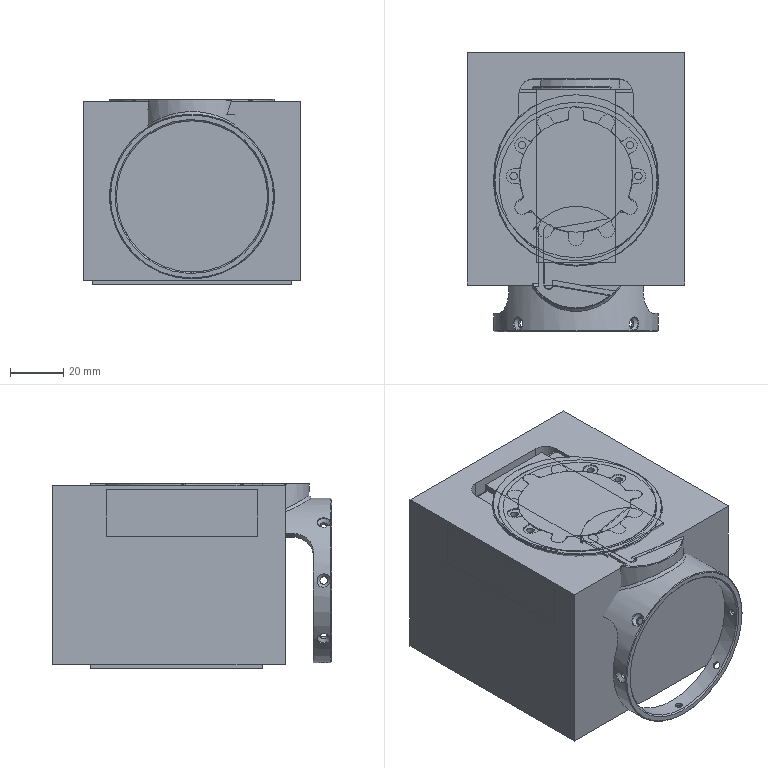NC program | NX | posted with a generic post | part box 82 x 105.2 x 70 mm
Lines 1141 to 2964 of 2964, first 1557 of 1814 lines:
(轮廓清角-D12 , TOOL : 光刀D2)
N2274 T22 M6
N2276 G53
N2278 G17 G0 G90 X21.079 Y-16.133 B0. C0. S8500 M3
N2280 G43 Z10. H22
N2282 Z-0.15
N2284 G41 G94 G1 X20.991 Y-15.953 F1000. D22
N2286 G3 X20.147 Y-15.394 R1.
N2288 G2 X18.452 Y-14.891 R3.8
N2290 G1 X17.13 Y-14.128
N2292 G2 X14.465 Y-16.822 R22.3
N2294 G3 X14.151 Y-17.854 R1.
N2296 G40
N2298 G1 X14.206 Y-18.047
N2300 G0 X21.079 Y-16.133 Z-0.3
N2302 G41 G1 X20.991 Y-15.953
N2304 G3 X20.147 Y-15.394 R1.
N2306 G2 X18.452 Y-14.891 R3.8
N2308 G1 X17.13 Y-14.128
N2310 G2 X14.465 Y-16.822 R22.3
N2312 G3 X14.151 Y-17.854 R1.
N2314 G40
N2316 G1 X14.206 Y-18.047
N2318 G0 X21.079 Y-16.133 Z-0.45
N2320 G41 G1 X20.991 Y-15.953
N2322 G3 X20.147 Y-15.394 R1.
N2324 G2 X18.452 Y-14.891 R3.8
N2326 G1 X17.13 Y-14.128
N2328 G2 X14.465 Y-16.822 R22.3
N2330 G3 X14.151 Y-17.854 R1.
N2332 G40
N2334 G1 X14.206 Y-18.047
N2336 G0 X21.079 Y-16.133 Z-0.6
N2338 G41 G1 X20.991 Y-15.953
N2340 G3 X20.147 Y-15.394 R1.
N2342 G2 X18.452 Y-14.891 R3.8
N2344 G1 X17.13 Y-14.128
N2346 G2 X14.465 Y-16.822 R22.3
N2348 G3 X14.151 Y-17.854 R1.
N2350 G40
N2352 G1 X14.206 Y-18.047
N2354 G0 X21.079 Y-16.133 Z-0.75
N2356 G41 G1 X20.991 Y-15.953
N2358 G3 X20.147 Y-15.394 R1.
N2360 G2 X18.452 Y-14.891 R3.8
N2362 G1 X17.13 Y-14.128
N2364 G2 X14.465 Y-16.822 R22.3
N2366 G3 X14.151 Y-17.854 R1.
N2368 G40
N2370 G1 X14.206 Y-18.047
N2372 G0 X21.079 Y-16.133 Z-0.9
N2374 G41 G1 X20.991 Y-15.953
N2376 G3 X20.147 Y-15.394 R1.
N2378 G2 X18.452 Y-14.891 R3.8
N2380 G1 X17.13 Y-14.128
N2382 G2 X14.465 Y-16.822 R22.3
N2384 G3 X14.151 Y-17.854 R1.
N2386 G40
N2388 G1 X14.206 Y-18.047
N2390 G0 X21.079 Y-16.133 Z-1.05
N2392 G41 G1 X20.991 Y-15.953
N2394 G3 X20.147 Y-15.394 R1.
N2396 G2 X18.452 Y-14.891 R3.8
N2398 G1 X17.13 Y-14.128
N2400 G2 X14.465 Y-16.822 R22.3
N2402 G3 X14.151 Y-17.854 R1.
N2404 G40
N2406 G1 X14.206 Y-18.047
N2408 G0 X21.079 Y-16.133 Z-1.2
N2410 G41 G1 X20.991 Y-15.953
N2412 G3 X20.147 Y-15.394 R1.
N2414 G2 X18.452 Y-14.891 R3.8
N2416 G1 X17.13 Y-14.128
N2418 G2 X14.465 Y-16.822 R22.3
N2420 G3 X14.151 Y-17.854 R1.
N2422 G40
N2424 G1 X14.206 Y-18.047
N2426 G0 X21.079 Y-16.133 Z-1.35
N2428 G41 G1 X20.991 Y-15.953
N2430 G3 X20.147 Y-15.394 R1.
N2432 G2 X18.452 Y-14.891 R3.8
N2434 G1 X17.13 Y-14.128
N2436 G2 X14.465 Y-16.822 R22.3
N2438 G3 X14.151 Y-17.854 R1.
N2440 G40
N2442 G1 X14.206 Y-18.047
N2444 G0 X21.079 Y-16.133 Z-1.5
N2446 G41 G1 X20.991 Y-15.953
N2448 G3 X20.147 Y-15.394 R1.
N2450 G2 X18.452 Y-14.891 R3.8
N2452 G1 X17.13 Y-14.128
N2454 G2 X14.465 Y-16.822 R22.3
N2456 G3 X14.151 Y-17.854 R1.
N2458 G40
N2460 G1 X14.206 Y-18.047
N2462 G0 X21.079 Y-16.133 Z-1.65
N2464 G41 G1 X20.991 Y-15.953
N2466 G3 X20.147 Y-15.394 R1.
N2468 G2 X18.452 Y-14.891 R3.8
N2470 G1 X17.13 Y-14.128
N2472 G2 X14.465 Y-16.822 R22.3
N2474 G3 X14.151 Y-17.854 R1.
N2476 G40
N2478 G1 X14.206 Y-18.047
N2480 G0 X21.079 Y-16.133 Z-1.8
N2482 G41 G1 X20.991 Y-15.953
N2484 G3 X20.147 Y-15.394 R1.
N2486 G2 X18.452 Y-14.891 R3.8
N2488 G1 X17.13 Y-14.128
N2490 G2 X14.465 Y-16.822 R22.3
N2492 G3 X14.151 Y-17.854 R1.
N2494 G40
N2496 G1 X14.206 Y-18.047
N2498 G0 X21.079 Y-16.133 Z-1.95
N2500 G41 G1 X20.991 Y-15.953
N2502 G3 X20.147 Y-15.394 R1.
N2504 G2 X18.452 Y-14.891 R3.8
N2506 G1 X17.13 Y-14.128
N2508 G2 X14.465 Y-16.822 R22.3
N2510 G3 X14.151 Y-17.854 R1.
N2512 G40
N2514 G1 X14.206 Y-18.047
N2516 G0 X21.079 Y-16.133 Z-2.1
N2518 G41 G1 X20.991 Y-15.953
N2520 G3 X20.147 Y-15.394 R1.
N2522 G2 X18.452 Y-14.891 R3.8
N2524 G1 X17.13 Y-14.128
N2526 G2 X14.465 Y-16.822 R22.3
N2528 G3 X14.151 Y-17.854 R1.
N2530 G40
N2532 G1 X14.206 Y-18.047
N2534 G0 X21.079 Y-16.133 Z-2.25
N2536 G41 G1 X20.991 Y-15.953
N2538 G3 X20.147 Y-15.394 R1.
N2540 G2 X18.452 Y-14.891 R3.8
N2542 G1 X17.13 Y-14.128
N2544 G2 X14.465 Y-16.822 R22.3
N2546 G3 X14.151 Y-17.854 R1.
N2548 G40
N2550 G1 X14.206 Y-18.047
N2552 G0 X21.079 Y-16.133 Z-2.4
N2554 G41 G1 X20.991 Y-15.953
N2556 G3 X20.147 Y-15.394 R1.
N2558 G2 X18.452 Y-14.891 R3.8
N2560 G1 X17.13 Y-14.128
N2562 G2 X14.465 Y-16.822 R22.3
N2564 G3 X14.151 Y-17.854 R1.
N2566 G40
N2568 G1 X14.206 Y-18.047
N2570 G0 X21.079 Y-16.133 Z-2.45
N2572 G41 G1 X20.991 Y-15.953
N2574 G3 X20.147 Y-15.394 R1.
N2576 G2 X18.452 Y-14.891 R3.8
N2578 G1 X17.13 Y-14.128
N2580 G2 X14.465 Y-16.822 R22.3
N2582 G3 X14.151 Y-17.854 R1.
N2584 G40
N2586 G1 X14.206 Y-18.047
N2588 G0 Z10.
N2590 X22.862 Y-3.054
N2592 Z-0.15
N2594 G41 G1 X22.668 Y-3.103
N2596 G3 X21.931 Y-3.891 R1.
N2598 G2 X20.93 Y-7.546 R22.3
N2600 G1 X22.252 Y-8.309
N2602 G2 X23.535 Y-9.526 R3.8
N2604 G3 X24.442 Y-9.977 R1.
N2606 G40
N2608 G1 X24.641 Y-9.964
N2610 G0 X22.862 Y-3.054 Z-0.3
N2612 G41 G1 X22.668 Y-3.103
N2614 G3 X21.931 Y-3.891 R1.
N2616 G2 X20.93 Y-7.546 R22.3
N2618 G1 X22.252 Y-8.309
N2620 G2 X23.535 Y-9.526 R3.8
N2622 G3 X24.442 Y-9.977 R1.
N2624 G40
N2626 G1 X24.641 Y-9.964
N2628 G0 X22.862 Y-3.054 Z-0.45
N2630 G41 G1 X22.668 Y-3.103
N2632 G3 X21.931 Y-3.891 R1.
N2634 G2 X20.93 Y-7.546 R22.3
N2636 G1 X22.252 Y-8.309
N2638 G2 X23.535 Y-9.526 R3.8
N2640 G3 X24.442 Y-9.977 R1.
N2642 G40
N2644 G1 X24.641 Y-9.964
N2646 G0 X22.862 Y-3.054 Z-0.6
N2648 G41 G1 X22.668 Y-3.103
N2650 G3 X21.931 Y-3.891 R1.
N2652 G2 X20.93 Y-7.546 R22.3
N2654 G1 X22.252 Y-8.309
N2656 G2 X23.535 Y-9.526 R3.8
N2658 G3 X24.442 Y-9.977 R1.
N2660 G40
N2662 G1 X24.641 Y-9.964
N2664 G0 X22.862 Y-3.054 Z-0.75
N2666 G41 G1 X22.668 Y-3.103
N2668 G3 X21.931 Y-3.891 R1.
N2670 G2 X20.93 Y-7.546 R22.3
N2672 G1 X22.252 Y-8.309
N2674 G2 X23.535 Y-9.526 R3.8
N2676 G3 X24.442 Y-9.977 R1.
N2678 G40
N2680 G1 X24.641 Y-9.964
N2682 G0 X22.862 Y-3.054 Z-0.9
N2684 G41 G1 X22.668 Y-3.103
N2686 G3 X21.931 Y-3.891 R1.
N2688 G2 X20.93 Y-7.546 R22.3
N2690 G1 X22.252 Y-8.309
N2692 G2 X23.535 Y-9.526 R3.8
N2694 G3 X24.442 Y-9.977 R1.
N2696 G40
N2698 G1 X24.641 Y-9.964
N2700 G0 X22.862 Y-3.054 Z-1.05
N2702 G41 G1 X22.668 Y-3.103
N2704 G3 X21.931 Y-3.891 R1.
N2706 G2 X20.93 Y-7.546 R22.3
N2708 G1 X22.252 Y-8.309
N2710 G2 X23.535 Y-9.526 R3.8
N2712 G3 X24.442 Y-9.977 R1.
N2714 G40
N2716 G1 X24.641 Y-9.964
N2718 G0 X22.862 Y-3.054 Z-1.2
N2720 G41 G1 X22.668 Y-3.103
N2722 G3 X21.931 Y-3.891 R1.
N2724 G2 X20.93 Y-7.546 R22.3
N2726 G1 X22.252 Y-8.309
N2728 G2 X23.535 Y-9.526 R3.8
N2730 G3 X24.442 Y-9.977 R1.
N2732 G40
N2734 G1 X24.641 Y-9.964
N2736 G0 X22.862 Y-3.054 Z-1.35
N2738 G41 G1 X22.668 Y-3.103
N2740 G3 X21.931 Y-3.891 R1.
N2742 G2 X20.93 Y-7.546 R22.3
N2744 G1 X22.252 Y-8.309
N2746 G2 X23.535 Y-9.526 R3.8
N2748 G3 X24.442 Y-9.977 R1.
N2750 G40
N2752 G1 X24.641 Y-9.964
N2754 G0 X22.862 Y-3.054 Z-1.5
N2756 G41 G1 X22.668 Y-3.103
N2758 G3 X21.931 Y-3.891 R1.
N2760 G2 X20.93 Y-7.546 R22.3
N2762 G1 X22.252 Y-8.309
N2764 G2 X23.535 Y-9.526 R3.8
N2766 G3 X24.442 Y-9.977 R1.
N2768 G40
N2770 G1 X24.641 Y-9.964
N2772 G0 X22.862 Y-3.054 Z-1.65
N2774 G41 G1 X22.668 Y-3.103
N2776 G3 X21.931 Y-3.891 R1.
N2778 G2 X20.93 Y-7.546 R22.3
N2780 G1 X22.252 Y-8.309
N2782 G2 X23.535 Y-9.526 R3.8
N2784 G3 X24.442 Y-9.977 R1.
N2786 G40
N2788 G1 X24.641 Y-9.964
N2790 G0 X22.862 Y-3.054 Z-1.8
N2792 G41 G1 X22.668 Y-3.103
N2794 G3 X21.931 Y-3.891 R1.
N2796 G2 X20.93 Y-7.546 R22.3
N2798 G1 X22.252 Y-8.309
N2800 G2 X23.535 Y-9.526 R3.8
N2802 G3 X24.442 Y-9.977 R1.
N2804 G40
N2806 G1 X24.641 Y-9.964
N2808 G0 X22.862 Y-3.054 Z-1.95
N2810 G41 G1 X22.668 Y-3.103
N2812 G3 X21.931 Y-3.891 R1.
N2814 G2 X20.93 Y-7.546 R22.3
N2816 G1 X22.252 Y-8.309
N2818 G2 X23.535 Y-9.526 R3.8
N2820 G3 X24.442 Y-9.977 R1.
N2822 G40
N2824 G1 X24.641 Y-9.964
N2826 G0 X22.862 Y-3.054 Z-2.1
N2828 G41 G1 X22.668 Y-3.103
N2830 G3 X21.931 Y-3.891 R1.
N2832 G2 X20.93 Y-7.546 R22.3
N2834 G1 X22.252 Y-8.309
N2836 G2 X23.535 Y-9.526 R3.8
N2838 G3 X24.442 Y-9.977 R1.
N2840 G40
N2842 G1 X24.641 Y-9.964
N2844 G0 X22.862 Y-3.054 Z-2.25
N2846 G41 G1 X22.668 Y-3.103
N2848 G3 X21.931 Y-3.891 R1.
N2850 G2 X20.93 Y-7.546 R22.3
N2852 G1 X22.252 Y-8.309
N2854 G2 X23.535 Y-9.526 R3.8
N2856 G3 X24.442 Y-9.977 R1.
N2858 G40
N2860 G1 X24.641 Y-9.964
N2862 G0 X22.862 Y-3.054 Z-2.4
N2864 G41 G1 X22.668 Y-3.103
N2866 G3 X21.931 Y-3.891 R1.
N2868 G2 X20.93 Y-7.546 R22.3
N2870 G1 X22.252 Y-8.309
N2872 G2 X23.535 Y-9.526 R3.8
N2874 G3 X24.442 Y-9.977 R1.
N2876 G40
N2878 G1 X24.641 Y-9.964
N2880 G0 X22.862 Y-3.054 Z-2.45
N2882 G41 G1 X22.668 Y-3.103
N2884 G3 X21.931 Y-3.891 R1.
N2886 G2 X20.93 Y-7.546 R22.3
N2888 G1 X22.252 Y-8.309
N2890 G2 X23.535 Y-9.526 R3.8
N2892 G3 X24.442 Y-9.977 R1.
N2894 G40
N2896 G1 X24.641 Y-9.964
N2898 G0 Z10.
N2900 X3.562 Y26.547
N2902 Z-0.15
N2904 G41 G1 X3.45 Y26.381
N2906 G3 X3.388 Y25.37 R1.
N2908 G2 X3.8 Y23.65 R3.8
N2910 G1 Y22.124
N2912 G2 X7.466 Y21.163 R22.3
N2914 G3 X8.516 Y21.408 R1.
N2916 G40
N2918 G1 X8.656 Y21.551
N2920 G0 X3.562 Y26.547 Z-0.3
N2922 G41 G1 X3.45 Y26.381
N2924 G3 X3.388 Y25.37 R1.
N2926 G2 X3.8 Y23.65 R3.8
N2928 G1 Y22.124
N2930 G2 X7.466 Y21.163 R22.3
N2932 G3 X8.516 Y21.408 R1.
N2934 G40
N2936 G1 X8.656 Y21.551
N2938 G0 X3.562 Y26.547 Z-0.45
N2940 G41 G1 X3.45 Y26.381
N2942 G3 X3.388 Y25.37 R1.
N2944 G2 X3.8 Y23.65 R3.8
N2946 G1 Y22.124
N2948 G2 X7.466 Y21.163 R22.3
N2950 G3 X8.516 Y21.408 R1.
N2952 G40
N2954 G1 X8.656 Y21.551
N2956 G0 X3.562 Y26.547 Z-0.6
N2958 G41 G1 X3.45 Y26.381
N2960 G3 X3.388 Y25.37 R1.
N2962 G2 X3.8 Y23.65 R3.8
N2964 G1 Y22.124
N2966 G2 X7.466 Y21.163 R22.3
N2968 G3 X8.516 Y21.408 R1.
N2970 G40
N2972 G1 X8.656 Y21.551
N2974 G0 X3.562 Y26.547 Z-0.75
N2976 G41 G1 X3.45 Y26.381
N2978 G3 X3.388 Y25.37 R1.
N2980 G2 X3.8 Y23.65 R3.8
N2982 G1 Y22.124
N2984 G2 X7.466 Y21.163 R22.3
N2986 G3 X8.516 Y21.408 R1.
N2988 G40
N2990 G1 X8.656 Y21.551
N2992 G0 X3.562 Y26.547 Z-0.9
N2994 G41 G1 X3.45 Y26.381
N2996 G3 X3.388 Y25.37 R1.
N2998 G2 X3.8 Y23.65 R3.8
N3000 G1 Y22.124
N3002 G2 X7.466 Y21.163 R22.3
N3004 G3 X8.516 Y21.408 R1.
N3006 G40
N3008 G1 X8.656 Y21.551
N3010 G0 X3.562 Y26.547 Z-1.05
N3012 G41 G1 X3.45 Y26.381
N3014 G3 X3.388 Y25.37 R1.
N3016 G2 X3.8 Y23.65 R3.8
N3018 G1 Y22.124
N3020 G2 X7.466 Y21.163 R22.3
N3022 G3 X8.516 Y21.408 R1.
N3024 G40
N3026 G1 X8.656 Y21.551
N3028 G0 X3.562 Y26.547 Z-1.2
N3030 G41 G1 X3.45 Y26.381
N3032 G3 X3.388 Y25.37 R1.
N3034 G2 X3.8 Y23.65 R3.8
N3036 G1 Y22.124
N3038 G2 X7.466 Y21.163 R22.3
N3040 G3 X8.516 Y21.408 R1.
N3042 G40
N3044 G1 X8.656 Y21.551
N3046 G0 X3.562 Y26.547 Z-1.35
N3048 G41 G1 X3.45 Y26.381
N3050 G3 X3.388 Y25.37 R1.
N3052 G2 X3.8 Y23.65 R3.8
N3054 G1 Y22.124
N3056 G2 X7.466 Y21.163 R22.3
N3058 G3 X8.516 Y21.408 R1.
N3060 G40
N3062 G1 X8.656 Y21.551
N3064 G0 X3.562 Y26.547 Z-1.5
N3066 G41 G1 X3.45 Y26.381
N3068 G3 X3.388 Y25.37 R1.
N3070 G2 X3.8 Y23.65 R3.8
N3072 G1 Y22.124
N3074 G2 X7.466 Y21.163 R22.3
N3076 G3 X8.516 Y21.408 R1.
N3078 G40
N3080 G1 X8.656 Y21.551
N3082 G0 X3.562 Y26.547 Z-1.65
N3084 G41 G1 X3.45 Y26.381
N3086 G3 X3.388 Y25.37 R1.
N3088 G2 X3.8 Y23.65 R3.8
N3090 G1 Y22.124
N3092 G2 X7.466 Y21.163 R22.3
N3094 G3 X8.516 Y21.408 R1.
N3096 G40
N3098 G1 X8.656 Y21.551
N3100 G0 X3.562 Y26.547 Z-1.8
N3102 G41 G1 X3.45 Y26.381
N3104 G3 X3.388 Y25.37 R1.
N3106 G2 X3.8 Y23.65 R3.8
N3108 G1 Y22.124
N3110 G2 X7.466 Y21.163 R22.3
N3112 G3 X8.516 Y21.408 R1.
N3114 G40
N3116 G1 X8.656 Y21.551
N3118 G0 X3.562 Y26.547 Z-1.95
N3120 G41 G1 X3.45 Y26.381
N3122 G3 X3.388 Y25.37 R1.
N3124 G2 X3.8 Y23.65 R3.8
N3126 G1 Y22.124
N3128 G2 X7.466 Y21.163 R22.3
N3130 G3 X8.516 Y21.408 R1.
N3132 G40
N3134 G1 X8.656 Y21.551
N3136 G0 X3.562 Y26.547 Z-2.1
N3138 G41 G1 X3.45 Y26.381
N3140 G3 X3.388 Y25.37 R1.
N3142 G2 X3.8 Y23.65 R3.8
N3144 G1 Y22.124
N3146 G2 X7.466 Y21.163 R22.3
N3148 G3 X8.516 Y21.408 R1.
N3150 G40
N3152 G1 X8.656 Y21.551
N3154 G0 X3.562 Y26.547 Z-2.25
N3156 G41 G1 X3.45 Y26.381
N3158 G3 X3.388 Y25.37 R1.
N3160 G2 X3.8 Y23.65 R3.8
N3162 G1 Y22.124
N3164 G2 X7.466 Y21.163 R22.3
N3166 G3 X8.516 Y21.408 R1.
N3168 G40
N3170 G1 X8.656 Y21.551
N3172 G0 X3.562 Y26.547 Z-2.4
N3174 G41 G1 X3.45 Y26.381
N3176 G3 X3.388 Y25.37 R1.
N3178 G2 X3.8 Y23.65 R3.8
N3180 G1 Y22.124
N3182 G2 X7.466 Y21.163 R22.3
N3184 G3 X8.516 Y21.408 R1.
N3186 G40
N3188 G1 X8.656 Y21.551
N3190 G0 X3.562 Y26.547 Z-2.45
N3192 G41 G1 X3.45 Y26.381
N3194 G3 X3.388 Y25.37 R1.
N3196 G2 X3.8 Y23.65 R3.8
N3198 G1 Y22.124
N3200 G2 X7.466 Y21.163 R22.3
N3202 G3 X8.516 Y21.408 R1.
N3204 G40
N3206 G1 X8.656 Y21.551
N3208 G0 Z10.
N3210 X-8.656
N3212 Z-0.15
N3214 G41 G1 X-8.516 Y21.408
N3216 G3 X-7.466 Y21.163 R1.
N3218 G2 X-3.8 Y22.124 R22.3
N3220 G1 Y23.65
N3222 G2 X-3.388 Y25.37 R3.8
N3224 G3 X-3.45 Y26.381 R1.
N3226 G40
N3228 G1 X-3.562 Y26.547
N3230 G0 X-8.656 Y21.551 Z-0.3
N3232 G41 G1 X-8.516 Y21.408
N3234 G3 X-7.466 Y21.163 R1.
N3236 G2 X-3.8 Y22.124 R22.3
N3238 G1 Y23.65
N3240 G2 X-3.388 Y25.37 R3.8
N3242 G3 X-3.45 Y26.381 R1.
N3244 G40
N3246 G1 X-3.562 Y26.547
N3248 G0 X-8.656 Y21.551 Z-0.45
N3250 G41 G1 X-8.516 Y21.408
N3252 G3 X-7.466 Y21.163 R1.
N3254 G2 X-3.8 Y22.124 R22.3
N3256 G1 Y23.65
N3258 G2 X-3.388 Y25.37 R3.8
N3260 G3 X-3.45 Y26.381 R1.
N3262 G40
N3264 G1 X-3.562 Y26.547
N3266 G0 X-8.656 Y21.551 Z-0.6
N3268 G41 G1 X-8.516 Y21.408
N3270 G3 X-7.466 Y21.163 R1.
N3272 G2 X-3.8 Y22.124 R22.3
N3274 G1 Y23.65
N3276 G2 X-3.388 Y25.37 R3.8
N3278 G3 X-3.45 Y26.381 R1.
N3280 G40
N3282 G1 X-3.562 Y26.547
N3284 G0 X-8.656 Y21.551 Z-0.75
N3286 G41 G1 X-8.516 Y21.408
N3288 G3 X-7.466 Y21.163 R1.
N3290 G2 X-3.8 Y22.124 R22.3
N3292 G1 Y23.65
N3294 G2 X-3.388 Y25.37 R3.8
N3296 G3 X-3.45 Y26.381 R1.
N3298 G40
N3300 G1 X-3.562 Y26.547
N3302 G0 X-8.656 Y21.551 Z-0.9
N3304 G41 G1 X-8.516 Y21.408
N3306 G3 X-7.466 Y21.163 R1.
N3308 G2 X-3.8 Y22.124 R22.3
N3310 G1 Y23.65
N3312 G2 X-3.388 Y25.37 R3.8
N3314 G3 X-3.45 Y26.381 R1.
N3316 G40
N3318 G1 X-3.562 Y26.547
N3320 G0 X-8.656 Y21.551 Z-1.05
N3322 G41 G1 X-8.516 Y21.408
N3324 G3 X-7.466 Y21.163 R1.
N3326 G2 X-3.8 Y22.124 R22.3
N3328 G1 Y23.65
N3330 G2 X-3.388 Y25.37 R3.8
N3332 G3 X-3.45 Y26.381 R1.
N3334 G40
N3336 G1 X-3.562 Y26.547
N3338 G0 X-8.656 Y21.551 Z-1.2
N3340 G41 G1 X-8.516 Y21.408
N3342 G3 X-7.466 Y21.163 R1.
N3344 G2 X-3.8 Y22.124 R22.3
N3346 G1 Y23.65
N3348 G2 X-3.388 Y25.37 R3.8
N3350 G3 X-3.45 Y26.381 R1.
N3352 G40
N3354 G1 X-3.562 Y26.547
N3356 G0 X-8.656 Y21.551 Z-1.35
N3358 G41 G1 X-8.516 Y21.408
N3360 G3 X-7.466 Y21.163 R1.
N3362 G2 X-3.8 Y22.124 R22.3
N3364 G1 Y23.65
N3366 G2 X-3.388 Y25.37 R3.8
N3368 G3 X-3.45 Y26.381 R1.
N3370 G40
N3372 G1 X-3.562 Y26.547
N3374 G0 X-8.656 Y21.551 Z-1.5
N3376 G41 G1 X-8.516 Y21.408
N3378 G3 X-7.466 Y21.163 R1.
N3380 G2 X-3.8 Y22.124 R22.3
N3382 G1 Y23.65
N3384 G2 X-3.388 Y25.37 R3.8
N3386 G3 X-3.45 Y26.381 R1.
N3388 G40
N3390 G1 X-3.562 Y26.547
N3392 G0 X-8.656 Y21.551 Z-1.65
N3394 G41 G1 X-8.516 Y21.408
N3396 G3 X-7.466 Y21.163 R1.
N3398 G2 X-3.8 Y22.124 R22.3
N3400 G1 Y23.65
N3402 G2 X-3.388 Y25.37 R3.8
N3404 G3 X-3.45 Y26.381 R1.
N3406 G40
N3408 G1 X-3.562 Y26.547
N3410 G0 X-8.656 Y21.551 Z-1.8
N3412 G41 G1 X-8.516 Y21.408
N3414 G3 X-7.466 Y21.163 R1.
N3416 G2 X-3.8 Y22.124 R22.3
N3418 G1 Y23.65
N3420 G2 X-3.388 Y25.37 R3.8
N3422 G3 X-3.45 Y26.381 R1.
N3424 G40
N3426 G1 X-3.562 Y26.547
N3428 G0 X-8.656 Y21.551 Z-1.95
N3430 G41 G1 X-8.516 Y21.408
N3432 G3 X-7.466 Y21.163 R1.
N3434 G2 X-3.8 Y22.124 R22.3
N3436 G1 Y23.65
N3438 G2 X-3.388 Y25.37 R3.8
N3440 G3 X-3.45 Y26.381 R1.
N3442 G40
N3444 G1 X-3.562 Y26.547
N3446 G0 X-8.656 Y21.551 Z-2.1
N3448 G41 G1 X-8.516 Y21.408
N3450 G3 X-7.466 Y21.163 R1.
N3452 G2 X-3.8 Y22.124 R22.3
N3454 G1 Y23.65
N3456 G2 X-3.388 Y25.37 R3.8
N3458 G3 X-3.45 Y26.381 R1.
N3460 G40
N3462 G1 X-3.562 Y26.547
N3464 G0 X-8.656 Y21.551 Z-2.25
N3466 G41 G1 X-8.516 Y21.408
N3468 G3 X-7.466 Y21.163 R1.
N3470 G2 X-3.8 Y22.124 R22.3
N3472 G1 Y23.65
N3474 G2 X-3.388 Y25.37 R3.8
N3476 G3 X-3.45 Y26.381 R1.
N3478 G40
N3480 G1 X-3.562 Y26.547
N3482 G0 X-8.656 Y21.551 Z-2.4
N3484 G41 G1 X-8.516 Y21.408
N3486 G3 X-7.466 Y21.163 R1.
N3488 G2 X-3.8 Y22.124 R22.3
N3490 G1 Y23.65
N3492 G2 X-3.388 Y25.37 R3.8
N3494 G3 X-3.45 Y26.381 R1.
N3496 G40
N3498 G1 X-3.562 Y26.547
N3500 G0 X-8.656 Y21.551 Z-2.45
N3502 G41 G1 X-8.516 Y21.408
N3504 G3 X-7.466 Y21.163 R1.
N3506 G2 X-3.8 Y22.124 R22.3
N3508 G1 Y23.65
N3510 G2 X-3.388 Y25.37 R3.8
N3512 G3 X-3.45 Y26.381 R1.
N3514 G40
N3516 G1 X-3.562 Y26.547
N3518 G0 Z10.
N3520 X-24.641 Y-9.964
N3522 Z-0.15
N3524 G41 G1 X-24.442 Y-9.977
N3526 G3 X-23.535 Y-9.526 R1.
N3528 G2 X-22.252 Y-8.309 R3.8
N3530 G1 X-20.93 Y-7.546
N3532 G2 X-21.931 Y-3.891 R22.3
N3534 G3 X-22.668 Y-3.103 R1.
N3536 G40
N3538 G1 X-22.862 Y-3.054
N3540 G0 X-24.641 Y-9.964 Z-0.3
N3542 G41 G1 X-24.442 Y-9.977
N3544 G3 X-23.535 Y-9.526 R1.
N3546 G2 X-22.252 Y-8.309 R3.8
N3548 G1 X-20.93 Y-7.546
N3550 G2 X-21.931 Y-3.891 R22.3
N3552 G3 X-22.668 Y-3.103 R1.
N3554 G40
N3556 G1 X-22.862 Y-3.054
N3558 G0 X-24.641 Y-9.964 Z-0.45
N3560 G41 G1 X-24.442 Y-9.977
N3562 G3 X-23.535 Y-9.526 R1.
N3564 G2 X-22.252 Y-8.309 R3.8
N3566 G1 X-20.93 Y-7.546
N3568 G2 X-21.931 Y-3.891 R22.3
N3570 G3 X-22.668 Y-3.103 R1.
N3572 G40
N3574 G1 X-22.862 Y-3.054
N3576 G0 X-24.641 Y-9.964 Z-0.6
N3578 G41 G1 X-24.442 Y-9.977
N3580 G3 X-23.535 Y-9.526 R1.
N3582 G2 X-22.252 Y-8.309 R3.8
N3584 G1 X-20.93 Y-7.546
N3586 G2 X-21.931 Y-3.891 R22.3
N3588 G3 X-22.668 Y-3.103 R1.
N3590 G40
N3592 G1 X-22.862 Y-3.054
N3594 G0 X-24.641 Y-9.964 Z-0.75
N3596 G41 G1 X-24.442 Y-9.977
N3598 G3 X-23.535 Y-9.526 R1.
N3600 G2 X-22.252 Y-8.309 R3.8
N3602 G1 X-20.93 Y-7.546
N3604 G2 X-21.931 Y-3.891 R22.3
N3606 G3 X-22.668 Y-3.103 R1.
N3608 G40
N3610 G1 X-22.862 Y-3.054
N3612 G0 X-24.641 Y-9.964 Z-0.9
N3614 G41 G1 X-24.442 Y-9.977
N3616 G3 X-23.535 Y-9.526 R1.
N3618 G2 X-22.252 Y-8.309 R3.8
N3620 G1 X-20.93 Y-7.546
N3622 G2 X-21.931 Y-3.891 R22.3
N3624 G3 X-22.668 Y-3.103 R1.
N3626 G40
N3628 G1 X-22.862 Y-3.054
N3630 G0 X-24.641 Y-9.964 Z-1.05
N3632 G41 G1 X-24.442 Y-9.977
N3634 G3 X-23.535 Y-9.526 R1.
N3636 G2 X-22.252 Y-8.309 R3.8
N3638 G1 X-20.93 Y-7.546
N3640 G2 X-21.931 Y-3.891 R22.3
N3642 G3 X-22.668 Y-3.103 R1.
N3644 G40
N3646 G1 X-22.862 Y-3.054
N3648 G0 X-24.641 Y-9.964 Z-1.2
N3650 G41 G1 X-24.442 Y-9.977
N3652 G3 X-23.535 Y-9.526 R1.
N3654 G2 X-22.252 Y-8.309 R3.8
N3656 G1 X-20.93 Y-7.546
N3658 G2 X-21.931 Y-3.891 R22.3
N3660 G3 X-22.668 Y-3.103 R1.
N3662 G40
N3664 G1 X-22.862 Y-3.054
N3666 G0 X-24.641 Y-9.964 Z-1.35
N3668 G41 G1 X-24.442 Y-9.977
N3670 G3 X-23.535 Y-9.526 R1.
N3672 G2 X-22.252 Y-8.309 R3.8
N3674 G1 X-20.93 Y-7.546
N3676 G2 X-21.931 Y-3.891 R22.3
N3678 G3 X-22.668 Y-3.103 R1.
N3680 G40
N3682 G1 X-22.862 Y-3.054
N3684 G0 X-24.641 Y-9.964 Z-1.5
N3686 G41 G1 X-24.442 Y-9.977
N3688 G3 X-23.535 Y-9.526 R1.
N3690 G2 X-22.252 Y-8.309 R3.8
N3692 G1 X-20.93 Y-7.546
N3694 G2 X-21.931 Y-3.891 R22.3
N3696 G3 X-22.668 Y-3.103 R1.
N3698 G40
N3700 G1 X-22.862 Y-3.054
N3702 G0 X-24.641 Y-9.964 Z-1.65
N3704 G41 G1 X-24.442 Y-9.977
N3706 G3 X-23.535 Y-9.526 R1.
N3708 G2 X-22.252 Y-8.309 R3.8
N3710 G1 X-20.93 Y-7.546
N3712 G2 X-21.931 Y-3.891 R22.3
N3714 G3 X-22.668 Y-3.103 R1.
N3716 G40
N3718 G1 X-22.862 Y-3.054
N3720 G0 X-24.641 Y-9.964 Z-1.8
N3722 G41 G1 X-24.442 Y-9.977
N3724 G3 X-23.535 Y-9.526 R1.
N3726 G2 X-22.252 Y-8.309 R3.8
N3728 G1 X-20.93 Y-7.546
N3730 G2 X-21.931 Y-3.891 R22.3
N3732 G3 X-22.668 Y-3.103 R1.
N3734 G40
N3736 G1 X-22.862 Y-3.054
N3738 G0 X-24.641 Y-9.964 Z-1.95
N3740 G41 G1 X-24.442 Y-9.977
N3742 G3 X-23.535 Y-9.526 R1.
N3744 G2 X-22.252 Y-8.309 R3.8
N3746 G1 X-20.93 Y-7.546
N3748 G2 X-21.931 Y-3.891 R22.3
N3750 G3 X-22.668 Y-3.103 R1.
N3752 G40
N3754 G1 X-22.862 Y-3.054
N3756 G0 X-24.641 Y-9.964 Z-2.1
N3758 G41 G1 X-24.442 Y-9.977
N3760 G3 X-23.535 Y-9.526 R1.
N3762 G2 X-22.252 Y-8.309 R3.8
N3764 G1 X-20.93 Y-7.546
N3766 G2 X-21.931 Y-3.891 R22.3
N3768 G3 X-22.668 Y-3.103 R1.
N3770 G40
N3772 G1 X-22.862 Y-3.054
N3774 G0 X-24.641 Y-9.964 Z-2.25
N3776 G41 G1 X-24.442 Y-9.977
N3778 G3 X-23.535 Y-9.526 R1.
N3780 G2 X-22.252 Y-8.309 R3.8
N3782 G1 X-20.93 Y-7.546
N3784 G2 X-21.931 Y-3.891 R22.3
N3786 G3 X-22.668 Y-3.103 R1.
N3788 G40
N3790 G1 X-22.862 Y-3.054
N3792 G0 X-24.641 Y-9.964 Z-2.4
N3794 G41 G1 X-24.442 Y-9.977
N3796 G3 X-23.535 Y-9.526 R1.
N3798 G2 X-22.252 Y-8.309 R3.8
N3800 G1 X-20.93 Y-7.546
N3802 G2 X-21.931 Y-3.891 R22.3
N3804 G3 X-22.668 Y-3.103 R1.
N3806 G40
N3808 G1 X-22.862 Y-3.054
N3810 G0 X-24.641 Y-9.964 Z-2.45
N3812 G41 G1 X-24.442 Y-9.977
N3814 G3 X-23.535 Y-9.526 R1.
N3816 G2 X-22.252 Y-8.309 R3.8
N3818 G1 X-20.93 Y-7.546
N3820 G2 X-21.931 Y-3.891 R22.3
N3822 G3 X-22.668 Y-3.103 R1.
N3824 G40
N3826 G1 X-22.862 Y-3.054
N3828 G0 Z10.
N3830 X-14.206 Y-18.047
N3832 Z-0.15
N3834 G41 G1 X-14.151 Y-17.854
N3836 G3 X-14.465 Y-16.822 R1.
N3838 G2 X-17.13 Y-14.128 R22.3
N3840 G1 X-18.452 Y-14.891
N3842 G2 X-20.147 Y-15.394 R3.8
N3844 G3 X-20.991 Y-15.953 R1.
N3846 G40
N3848 G1 X-21.079 Y-16.133
N3850 G0 X-14.206 Y-18.047 Z-0.3
N3852 G41 G1 X-14.151 Y-17.854
N3854 G3 X-14.465 Y-16.822 R1.
N3856 G2 X-17.13 Y-14.128 R22.3
N3858 G1 X-18.452 Y-14.891
N3860 G2 X-20.147 Y-15.394 R3.8
N3862 G3 X-20.991 Y-15.953 R1.
N3864 G40
N3866 G1 X-21.079 Y-16.133
N3868 G0 X-14.206 Y-18.047 Z-0.45
N3870 G41 G1 X-14.151 Y-17.854
N3872 G3 X-14.465 Y-16.822 R1.
N3874 G2 X-17.13 Y-14.128 R22.3
N3876 G1 X-18.452 Y-14.891
N3878 G2 X-20.147 Y-15.394 R3.8
N3880 G3 X-20.991 Y-15.953 R1.
N3882 G40
N3884 G1 X-21.079 Y-16.133
N3886 G0 X-14.206 Y-18.047 Z-0.6
N3888 G41 G1 X-14.151 Y-17.854
N3890 G3 X-14.465 Y-16.822 R1.
N3892 G2 X-17.13 Y-14.128 R22.3
N3894 G1 X-18.452 Y-14.891
N3896 G2 X-20.147 Y-15.394 R3.8
N3898 G3 X-20.991 Y-15.953 R1.
N3900 G40
N3902 G1 X-21.079 Y-16.133
N3904 G0 X-14.206 Y-18.047 Z-0.75
N3906 G41 G1 X-14.151 Y-17.854
N3908 G3 X-14.465 Y-16.822 R1.
N3910 G2 X-17.13 Y-14.128 R22.3
N3912 G1 X-18.452 Y-14.891
N3914 G2 X-20.147 Y-15.394 R3.8
N3916 G3 X-20.991 Y-15.953 R1.
N3918 G40
N3920 G1 X-21.079 Y-16.133
N3922 G0 X-14.206 Y-18.047 Z-0.9
N3924 G41 G1 X-14.151 Y-17.854
N3926 G3 X-14.465 Y-16.822 R1.
N3928 G2 X-17.13 Y-14.128 R22.3
N3930 G1 X-18.452 Y-14.891
N3932 G2 X-20.147 Y-15.394 R3.8
N3934 G3 X-20.991 Y-15.953 R1.
N3936 G40
N3938 G1 X-21.079 Y-16.133
N3940 G0 X-14.206 Y-18.047 Z-1.05
N3942 G41 G1 X-14.151 Y-17.854
N3944 G3 X-14.465 Y-16.822 R1.
N3946 G2 X-17.13 Y-14.128 R22.3
N3948 G1 X-18.452 Y-14.891
N3950 G2 X-20.147 Y-15.394 R3.8
N3952 G3 X-20.991 Y-15.953 R1.
N3954 G40
N3956 G1 X-21.079 Y-16.133
N3958 G0 X-14.206 Y-18.047 Z-1.2
N3960 G41 G1 X-14.151 Y-17.854
N3962 G3 X-14.465 Y-16.822 R1.
N3964 G2 X-17.13 Y-14.128 R22.3
N3966 G1 X-18.452 Y-14.891
N3968 G2 X-20.147 Y-15.394 R3.8
N3970 G3 X-20.991 Y-15.953 R1.
N3972 G40
N3974 G1 X-21.079 Y-16.133
N3976 G0 X-14.206 Y-18.047 Z-1.35
N3978 G41 G1 X-14.151 Y-17.854
N3980 G3 X-14.465 Y-16.822 R1.
N3982 G2 X-17.13 Y-14.128 R22.3
N3984 G1 X-18.452 Y-14.891
N3986 G2 X-20.147 Y-15.394 R3.8
N3988 G3 X-20.991 Y-15.953 R1.
N3990 G40
N3992 G1 X-21.079 Y-16.133
N3994 G0 X-14.206 Y-18.047 Z-1.5
N3996 G41 G1 X-14.151 Y-17.854
N3998 G3 X-14.465 Y-16.822 R1.
N4000 G2 X-17.13 Y-14.128 R22.3
N4002 G1 X-18.452 Y-14.891
N4004 G2 X-20.147 Y-15.394 R3.8
N4006 G3 X-20.991 Y-15.953 R1.
N4008 G40
N4010 G1 X-21.079 Y-16.133
N4012 G0 X-14.206 Y-18.047 Z-1.65
N4014 G41 G1 X-14.151 Y-17.854
N4016 G3 X-14.465 Y-16.822 R1.
N4018 G2 X-17.13 Y-14.128 R22.3
N4020 G1 X-18.452 Y-14.891
N4022 G2 X-20.147 Y-15.394 R3.8
N4024 G3 X-20.991 Y-15.953 R1.
N4026 G40
N4028 G1 X-21.079 Y-16.133
N4030 G0 X-14.206 Y-18.047 Z-1.8
N4032 G41 G1 X-14.151 Y-17.854
N4034 G3 X-14.465 Y-16.822 R1.
N4036 G2 X-17.13 Y-14.128 R22.3
N4038 G1 X-18.452 Y-14.891
N4040 G2 X-20.147 Y-15.394 R3.8
N4042 G3 X-20.991 Y-15.953 R1.
N4044 G40
N4046 G1 X-21.079 Y-16.133
N4048 G0 X-14.206 Y-18.047 Z-1.95
N4050 G41 G1 X-14.151 Y-17.854
N4052 G3 X-14.465 Y-16.822 R1.
N4054 G2 X-17.13 Y-14.128 R22.3
N4056 G1 X-18.452 Y-14.891
N4058 G2 X-20.147 Y-15.394 R3.8
N4060 G3 X-20.991 Y-15.953 R1.
N4062 G40
N4064 G1 X-21.079 Y-16.133
N4066 G0 X-14.206 Y-18.047 Z-2.1
N4068 G41 G1 X-14.151 Y-17.854
N4070 G3 X-14.465 Y-16.822 R1.
N4072 G2 X-17.13 Y-14.128 R22.3
N4074 G1 X-18.452 Y-14.891
N4076 G2 X-20.147 Y-15.394 R3.8
N4078 G3 X-20.991 Y-15.953 R1.
N4080 G40
N4082 G1 X-21.079 Y-16.133
N4084 G0 X-14.206 Y-18.047 Z-2.25
N4086 G41 G1 X-14.151 Y-17.854
N4088 G3 X-14.465 Y-16.822 R1.
N4090 G2 X-17.13 Y-14.128 R22.3
N4092 G1 X-18.452 Y-14.891
N4094 G2 X-20.147 Y-15.394 R3.8
N4096 G3 X-20.991 Y-15.953 R1.
N4098 G40
N4100 G1 X-21.079 Y-16.133
N4102 G0 X-14.206 Y-18.047 Z-2.4
N4104 G41 G1 X-14.151 Y-17.854
N4106 G3 X-14.465 Y-16.822 R1.
N4108 G2 X-17.13 Y-14.128 R22.3
N4110 G1 X-18.452 Y-14.891
N4112 G2 X-20.147 Y-15.394 R3.8
N4114 G3 X-20.991 Y-15.953 R1.
N4116 G40
N4118 G1 X-21.079 Y-16.133
N4120 G0 X-14.206 Y-18.047 Z-2.45
N4122 G41 G1 X-14.151 Y-17.854
N4124 G3 X-14.465 Y-16.822 R1.
N4126 G2 X-17.13 Y-14.128 R22.3
N4128 G1 X-18.452 Y-14.891
N4130 G2 X-20.147 Y-15.394 R3.8
N4132 G3 X-20.991 Y-15.953 R1.
N4134 G40
N4136 G1 X-21.079 Y-16.133
N4138 G0 Z10.
N4140 M5
(底壁铣选底_2 , TOOL : 光刀D10)
N4142 T10 M6
N4144 G53
N4146 G17 G0 G90 X-9.223 Y25.792 B0. C0. S8000 M3
N4148 G43 Z10. H10
N4150 Z1.
N4152 G94 G1 Z0. F1200.
N4154 X-8.764 Y24.516
N4156 G3 X-7.576 Y25.283 R1.
N4158 G2 X7.576 Y25.283 R7.75
N4160 X25.554 Y-5.855 R26.25
N4162 X17.978 Y-18.978 R7.75
N4164 X-17.978 Y-18.978 R26.25
N4166 X-25.554 Y-5.855 R7.75
N4168 X-7.576 Y25.283 R26.25
N4170 G1 X-4.001 Y21.788
N4172 G3 X-2.688 Y24.229 R5.
N4174 G2 X2.688 Y24.229 R2.75
N4176 G3 X6.133 Y20.496 R5.
N4178 G2 X20.686 Y-4.712 R21.25
N4180 G3 X22.198 Y-9.562 R5.
N4182 G2 X19.509 Y-14.218 R2.75
N4184 G3 X14.553 Y-15.334 R5.
N4186 G2 X-14.553 Y-15.334 R21.25
N4188 G3 X-19.509 Y-14.218 R5.
N4190 G2 X-22.198 Y-9.562 R2.75
N4192 G3 X-20.686 Y-4.712 R5.
N4194 G2 X-6.133 Y20.496 R21.25
N4196 G3 X-4.001 Y21.788 R5.
N4198 G1 X-0.426 Y18.292
N4200 G3 X0. Y18.756 R10.
N4202 X4.69 Y15.709 R10.
N4204 G2 X15.819 Y-3.568 R16.25
N4206 G3 X16.113 Y-9.153 R10.
N4208 X11.129 Y-11.691 R10.
N4210 G2 X-11.129 Y-11.691 R16.25
N4212 G3 X-16.113 Y-9.153 R10.
N4214 X-15.819 Y-3.568 R10.
N4216 G2 X-4.69 Y15.709 R16.25
N4218 G3 X-0.426 Y18.292 R10.
N4220 G1 X0. Y12.337
N4222 G3 X3.247 Y10.921 R15.
N4224 G2 X10.952 Y-2.424 R11.25
N4226 G3 X10.554 Y-5.943 R15.
N4228 X7.705 Y-8.048 R15.
N4230 G2 X-7.705 Y-8.048 R11.25
N4232 G3 X-10.554 Y-5.943 R15.
N4234 X-10.952 Y-2.424 R15.
N4236 G2 X-3.247 Y10.921 R11.25
N4238 G3 X0. Y12.337 R15.
N4240 G1 Y6.773
N4242 G3 X1.804 Y6.134 R20.
N4244 G2 X6.084 Y-1.28 R6.25
N4246 G3 X5.736 Y-3.162 R20.
N4248 X4.281 Y-4.404 R20.
N4250 G2 X-4.28 Y-4.404 R6.25
N4252 G3 X-5.736 Y-3.162 R20.
N4254 X-6.084 Y-1.28 R20.
N4256 G2 X-1.804 Y6.134 R6.25
N4258 G3 X0. Y6.773 R20.
N4260 G1 Y1.459
N4262 G3 X0.361 Y1.347 R25.
N4264 G2 X1.217 Y-0.136 R1.25
N4266 G3 X1.133 Y-0.504 R25.
N4268 X0.856 Y-0.76 R25.
N4270 G2 X-0.856 Y-0.761 R1.25
N4272 G3 X-1.133 Y-0.504 R25.
N4274 X-1.217 Y-0.136 R25.
N4276 G2 X-0.361 Y1.347 R1.25
N4278 G3 X0. Y1.459 R25.
N4280 X0.361 Y1.347 R25.
N4282 G2 X0.889 Y1.029 R1.25
N4284 G3 X2.303 Y1.022 R1.
N4286 G1 Z1.
N4288 G0 Z10.
N4290 X47.338 Y22.289
N4292 Z-1.5
N4294 G1 Z-2.5
N4296 G2 X46. Y22.746 R1.
N4298 G3 X36.128 Y36.5 R51.25
N4300 G1 X28.596
N4302 G2 X46. Y4.952 R46.25
N4304 G3 X47.098 Y4.062 R1.
N4306 G1 Z-1.5
N4308 G0 Z10.
N4310 X41.514 Y-37.91
N4312 Z-1.5
N4314 G1 Z-2.5
N4316 G2 X41.625 Y-36.5 R1.
N4318 G3 X46. Y-31.965 R32.75
N4320 G1 Y-30.5
N4322 Y-22.193
N4324 G2 X32.601 Y-36.5 R27.75
N4326 G1 X18.93
N4328 G3 X22.815 Y-34.216 R41.25
N4330 X41.17 Y-2.425 R22.75
N4332 X19.5 Y36.5 R41.25
N4334 G2 X19.091 Y37.854 R1.
N4336 G1 Z-1.5
N4338 G0 Z10.
N4340 X-36.124 Y37.914
N4342 Z-1.5
N4344 G1 Z-2.5
N4346 G2 X-36.128 Y36.5 R1.
N4348 G3 X-46. Y22.746 R51.25
N4350 G1 Y4.952
N4352 G2 X-28.596 Y36.5 R46.25
N4354 G3 X-28.429 Y37.904 R1.
N4356 G1 Z-1.5
N4358 G0 Z10.
N4360 X-47.405 Y-31.803
N4362 Z-1.5
N4364 G1 Z-2.5
N4366 G2 X-46. Y-31.965 R1.
N4368 G3 X-41.625 Y-36.5 R32.75
N4370 G1 X-32.601
N4372 G2 X-46. Y-22.193 R27.75
N4374 G3 X-47.306 Y-21.651 R1.
N4376 G1 Z-1.5
N4378 G0 Z10.
N4380 X-19.091 Y37.854
N4382 Z-1.5
N4384 G1 Z-2.5
N4386 G2 X-19.5 Y36.5 R1.
N4388 G3 X-41.17 Y-2.425 R41.25
N4390 X-22.815 Y-34.216 R22.75
N4392 X-18.93 Y-36.5 R41.25
N4394 G2 X-18.5 Y-37.847 R1.
N4396 G1 Z-1.5
N4398 G0 Z10.
N4400 X12.211 Y37.914
N4402 Z-1.5
N4404 G1 Z-2.5
N4406 G3 X12.245 Y36.5 R1.
N4408 G2 X14.99 Y33.155 R17.75
N4410 X36.079 Y-3.371 R36.25
N4412 X21.088 Y-29.335 R17.75
N4414 X-21.088 Y-29.335 R36.25
N4416 X-36.079 Y-3.371 R17.75
N4418 X-14.99 Y33.155 R36.25
N4420 X-12.245 Y36.5 R17.75
N4422 G1 X-8.796 Y32.88
N4424 G2 X11.469 Y29.219 R12.75
N4426 X30.909 Y-4.452 R31.25
N4428 X19.44 Y-24.317 R12.75
N4430 X-19.44 Y-24.317 R31.25
N4432 X-30.909 Y-4.452 R12.75
N4434 X-11.469 Y29.219 R31.25
N4436 X-8.796 Y32.88 R12.75
N4438 G1 X-5.346 Y29.261
N4440 G2 X7.576 Y25.283 R7.75
N4442 X25.554 Y-5.855 R26.25
N4444 X17.978 Y-18.978 R7.75
N4446 X-17.978 Y-18.978 R26.25
N4448 X-25.554 Y-5.855 R7.75
N4450 X-7.576 Y25.283 R26.25
N4452 X-5.346 Y29.261 R7.75
N4454 X-4.58 Y29.902 R7.75
N4456 G3 X-4.364 Y31.3 R1.
N4458 G1 Z-1.5
N4460 G0 Z10.
(单向轮廓精光_10 , TOOL : 光刀D10)
N4462 X46.52 Y-36.605
N4464 Z-17.5
N4466 G1 Z-20.5
N4468 G41 X44.964 Y-35.05 D10
N4470 G3 X43.55 Y-35.05 R1.
N4472 G2 X40. Y-36.52 R5.02
N4474 G1 X-40.
N4476 G2 X-43.55 Y-35.05 R5.02
N4478 G1 X-44.55 Y-34.05
N4480 G2 X-46.02 Y-30.5 R5.02
N4482 G1 Y26.5
N4484 G2 X-44.55 Y30.05 R5.02
N4486 G1 X-39.55 Y35.05
N4488 G2 X-36. Y36.52 R5.02
N4490 G1 X36.
N4492 G2 X39.55 Y35.05 R5.02
N4494 G1 X44.55 Y30.05
N4496 G2 X46.02 Y26.5 R5.02
N4498 G1 Y-30.5
N4500 G2 X44.55 Y-34.05 R5.02
N4502 G1 X43.55 Y-35.05
N4504 G2 X43.179 Y-35.385 R5.02
N4506 G3 X43.038 Y-36.792 R1.
N4508 G40
N4510 G1 X43.165 Y-36.947
N4512 X45.091 Y-35.177
N4514 G41 X44.95 Y-35.036
N4516 G3 X43.536 Y-35.036 R1.
N4518 G2 X40. Y-36.5 R5.
N4520 G1 X-40.
N4522 G2 X-43.536 Y-35.036 R5.
N4524 G1 X-44.536 Y-34.036
N4526 G2 X-46. Y-30.5 R5.
N4528 G1 Y26.5
N4530 G2 X-44.536 Y30.036 R5.
N4532 G1 X-39.536 Y35.036
N4534 G2 X-36. Y36.5 R5.
N4536 G1 X36.
N4538 G2 X39.536 Y35.036 R5.
N4540 G1 X44.536 Y30.036
N4542 G2 X46. Y26.5 R5.
N4544 G1 Y-30.5
N4546 G2 X44.536 Y-34.036 R5.
N4548 G1 X43.536 Y-35.036
N4550 G2 X43.165 Y-35.371 R5.
N4552 G3 X43.024 Y-36.778 R1.
N4554 G1 X44.263 Y-38.293
N4556 G40
N4558 X44.389 Y-38.448
N4560 Z-17.5
N4562 G0 Z10.
N4564 M5
(3轴去毛刺D6_1 , TOOL : 倒角刀D6)
N4566 T11 M6
N4568 G53
N4570 G17 G0 G90 X1.916 Y-23.521 B0. C0. S8000 M3
N4572 G43 Z5. H11
N4574 Z0.223
N4576 G94 G1 X1.915 Y-23.504 Z0.007 F900.
N4578 X1.913 Y-23.454 Z-0.205
N4580 X1.911 Y-23.377 Z-0.413
N4582 X1.907 Y-23.277 Z-0.613
N4584 X1.903 Y-23.157 Z-0.806
N4586 X1.899 Y-23.023 Z-0.99
N4588 X1.889 Y-22.726 Z-1.322
N4590 X1.879 Y-22.668 Z-1.381
N4592 X1.855 Y-22.613 Z-1.437
N4594 X1.77 Y-22.512 Z-1.54
N4596 X1.642 Y-22.426 Z-1.63
N4598 X1.483 Y-22.354 Z-1.707
N4600 X1.304 Y-22.298 Z-1.769
N4602 X1.114 Y-22.258 Z-1.815
N4604 X0.925 Y-22.236 Z-1.843
N4606 X0.747 Y-22.232 Z-1.853
N4608 X0.357 Y-22.244 F1000.
N4610 X0.247
N4612 X-0.357
N4614 X-1.072 Y-22.221
N4616 X-1.785 Y-22.176
N4618 X-2.497 Y-22.107
N4620 X-3.206 Y-22.016
N4622 X-3.912 Y-21.903
N4624 X-4.614 Y-21.766
N4626 X-5.311 Y-21.608
N4628 X-6.003 Y-21.427
N4630 X-6.688 Y-21.225
N4632 X-7.367 Y-21.
N4634 X-8.039 Y-20.754
N4636 X-8.702 Y-20.487
N4638 X-9.357 Y-20.199
N4640 X-10.001 Y-19.89
N4642 X-10.636 Y-19.56
N4644 X-11.26 Y-19.211
N4646 X-11.872 Y-18.842
N4648 X-12.472 Y-18.453
N4650 X-13.059 Y-18.046
N4652 X-13.633 Y-17.619
N4654 X-14.193 Y-17.176
N4656 X-14.738 Y-16.714
N4658 X-15.269 Y-16.236
N4660 X-15.784 Y-15.74
N4662 X-16.283 Y-15.228
N4664 X-16.765 Y-14.701
N4666 X-17.153 Y-14.25 Z-1.851
N4668 X-17.15 Y-14.251
N4670 X-18.446 Y-15. Z-1.852
N4672 X-18.718 Y-15.138 Z-1.853
N4674 X-19.039 Y-15.27
N4676 X-19.371 Y-15.373
N4678 X-19.713 Y-15.446 Z-1.854
N4680 X-20.06 Y-15.488 Z-1.853
N4682 X-20.409 Y-15.497
N4684 X-20.758 Y-15.477
N4686 X-21.104 Y-15.424
N4688 X-21.443 Y-15.341
N4690 X-21.774 Y-15.228
N4692 X-22.094 Y-15.086
N4694 X-22.4 Y-14.916
N4696 X-22.689 Y-14.719 Z-1.852
N4698 X-22.959 Y-14.496
N4700 X-23.208 Y-14.251
N4702 X-23.434 Y-13.984
N4704 X-23.636 Y-13.698
N4706 X-23.811 Y-13.395
N4708 X-23.958 Y-13.078
N4710 X-24.076 Y-12.749
N4712 X-24.164 Y-12.41
N4714 X-24.221 Y-12.065
N4716 X-24.247 Y-11.716 Z-1.853
N4718 X-24.242 Y-11.366
N4720 X-24.205 Y-11.018
N4722 X-24.138 Y-10.675
N4724 X-24.04 Y-10.339
N4726 X-23.912 Y-10.014
N4728 X-23.756 Y-9.701
N4730 X-23.573 Y-9.404
N4732 X-23.363 Y-9.124 Z-1.854
N4734 X-23.129 Y-8.864 Z-1.853
N4736 X-22.873 Y-8.628
N4738 X-22.599 Y-8.417
N4740 X-22.343 Y-8.25 Z-1.852
N4742 X-21.047 Y-7.501 Z-1.851
N4744 X-21.08 Y-7.41 Z-1.852
N4746 X-21.244 Y-6.944 Z-1.853
N4748 X-21.459 Y-6.262
N4750 X-21.653 Y-5.574
N4752 X-21.825 Y-4.88
N4754 X-21.974 Y-4.182
N4756 X-22.101 Y-3.479
N4758 X-22.206 Y-2.772
N4760 X-22.287 Y-2.062
N4762 X-22.347 Y-1.349
N4764 X-22.383 Y-0.636
N4766 X-22.397 Y0.079
N4768 X-22.388 Y0.794
N4770 X-22.356 Y1.508
N4772 X-22.301 Y2.221
N4774 X-22.223 Y2.932
N4776 X-22.123 Y3.64
N4778 X-22.001 Y4.345
N4780 X-21.855 Y5.045
N4782 X-21.688 Y5.74
N4784 X-21.499 Y6.43
N4786 X-21.287 Y7.112
N4788 X-21.054 Y7.788
N4790 X-20.8 Y8.456
N4792 X-20.524 Y9.116
N4794 X-20.227 Y9.767
N4796 X-19.91 Y10.407
N4798 X-19.573 Y11.037
N4800 X-19.215 Y11.657
N4802 X-18.838 Y12.264
N4804 X-18.442 Y12.859
N4806 X-18.027 Y13.441
N4808 X-17.593 Y14.01
N4810 X-17.142 Y14.564
N4812 X-16.673 Y15.104
N4814 X-16.187 Y15.629
N4816 X-15.685 Y16.137
N4818 X-15.167 Y16.63
N4820 X-14.633 Y17.106
N4822 X-14.084 Y17.564
N4824 X-13.521 Y18.005
N4826 X-12.944 Y18.428
N4828 X-12.354 Y18.831
N4830 X-11.752 Y19.216
N4832 X-11.137 Y19.582
N4834 X-10.511 Y19.927
N4836 X-9.875 Y20.253
N4838 X-9.228 Y20.557
N4840 X-8.572 Y20.842
N4842 X-7.908 Y21.105
N4844 X-7.236 Y21.346
N4846 X-6.556 Y21.566
N4848 X-5.869 Y21.764
N4850 X-5.177 Y21.94
N4852 X-4.479 Y22.095
N4854 X-3.993 Y22.185
N4856 X-3.898 Y22.206 Z-1.854
N4858 X-3.896 Y22.303 Z-1.852
N4860 X-3.897 Y23.7
N4862 X-3.881 Y24.005 Z-1.853
N4864 X-3.835 Y24.348
N4866 X-3.758 Y24.688
N4868 X-3.65 Y25.02 Z-1.854
N4870 X-3.513 Y25.341 Z-1.853
N4872 X-3.346 Y25.649
N4874 X-3.154 Y25.94
N4876 X-2.936 Y26.214
N4878 X-2.694 Y26.466
N4880 X-2.431 Y26.696
N4882 X-2.148 Y26.902
N4884 X-1.847 Y27.081
N4886 X-1.532 Y27.233 Z-1.852
N4888 X-1.205 Y27.356
N4890 X-0.867 Y27.449
N4892 X-0.523 Y27.512
N4894 X-0.175 Y27.543
N4896 X0.175
N4898 X0.523 Y27.512
N4900 X0.867 Y27.449
N4902 X1.205 Y27.356
N4904 X1.532 Y27.233
N4906 X1.847 Y27.081 Z-1.853
N4908 X2.148 Y26.902
N4910 X2.431 Y26.696
N4912 X2.694 Y26.466
N4914 X2.936 Y26.214
N4916 X3.154 Y25.94
N4918 X3.346 Y25.649
N4920 X3.512 Y25.341
N4922 X3.65 Y25.02 Z-1.854
N4924 X3.758 Y24.688 Z-1.853
N4926 X3.835 Y24.348
N4928 X3.881 Y24.005
N4930 X3.897 Y23.7 Z-1.852
N4932 X3.896 Y22.317
N4934 X3.952 Y22.25 Z-1.853
N4936 X4.007 Y22.184 Z-1.852
N4938 X4.479 Y22.095 Z-1.853
N4940 X5.177 Y21.94
N4942 X5.869 Y21.764
N4944 X6.556 Y21.566
N4946 X7.236 Y21.346
N4948 X7.908 Y21.105
N4950 X8.572 Y20.842
N4952 X9.228 Y20.557
N4954 X9.875 Y20.253
N4956 X10.511 Y19.927
N4958 X11.137 Y19.582
N4960 X11.752 Y19.216
N4962 X12.354 Y18.831
N4964 X12.944 Y18.428
N4966 X13.521 Y18.005
N4968 X14.084 Y17.564
N4970 X14.633 Y17.106
N4972 X15.167 Y16.63
N4974 X15.685 Y16.137
N4976 X16.187 Y15.629
N4978 X16.673 Y15.104
N4980 X17.142 Y14.564
N4982 X17.593 Y14.01
N4984 X18.027 Y13.441
N4986 X18.442 Y12.859
N4988 X18.838 Y12.264
N4990 X19.215 Y11.657
N4992 X19.573 Y11.037
N4994 X19.91 Y10.407
N4996 X20.227 Y9.767
N4998 X20.524 Y9.116
N5000 X20.8 Y8.456
N5002 X21.054 Y7.788
N5004 X21.287 Y7.112
N5006 X21.499 Y6.43
N5008 X21.688 Y5.74
N5010 X21.855 Y5.045
N5012 X22.001 Y4.345
N5014 X22.123 Y3.64
N5016 X22.223 Y2.932
N5018 X22.301 Y2.221
N5020 X22.356 Y1.508
N5022 X22.388 Y0.794
N5024 X22.397 Y0.079
N5026 X22.383 Y-0.636
N5028 X22.347 Y-1.349
N5030 X22.287 Y-2.062
N5032 X22.206 Y-2.772
N5034 X22.101 Y-3.479
N5036 X21.974 Y-4.182
N5038 X21.825 Y-4.88
N5040 X21.653 Y-5.574
N5042 X21.459 Y-6.262
N5044 X21.244 Y-6.944
N5046 X21.048 Y-7.505 Z-1.851
N5048 X21.133 Y-7.553 Z-1.852
N5050 X22.343 Y-8.25
N5052 X22.599 Y-8.417 Z-1.853
N5054 X22.873 Y-8.628
N5056 X23.129 Y-8.864
N5058 X23.363 Y-9.124 Z-1.854
N5060 X23.573 Y-9.404 Z-1.853
N5062 X23.756 Y-9.701
N5064 X23.912 Y-10.014
N5066 X24.04 Y-10.339
N5068 X24.138 Y-10.675
N5070 X24.205 Y-11.018
N5072 X24.242 Y-11.366
N5074 X24.247 Y-11.716
N5076 X24.221 Y-12.065 Z-1.852
N5078 X24.164 Y-12.41
N5080 X24.076 Y-12.749
N5082 X23.958 Y-13.078
N5084 X23.811 Y-13.395
N5086 X23.636 Y-13.698
N5088 X23.434 Y-13.984
N5090 X23.208 Y-14.251
N5092 X22.959 Y-14.496
N5094 X22.689 Y-14.719
N5096 X22.4 Y-14.916 Z-1.853
N5098 X22.094 Y-15.086
N5100 X21.774 Y-15.228
N5102 X21.443 Y-15.341
N5104 X21.104 Y-15.424
N5106 X20.758 Y-15.477
N5108 X20.409 Y-15.497
N5110 X20.06 Y-15.488
N5112 X19.713 Y-15.446 Z-1.854
N5114 X19.371 Y-15.373 Z-1.853
N5116 X19.039 Y-15.27
N5118 X18.718 Y-15.138
N5120 X18.446 Y-15. Z-1.852
N5122 X17.237 Y-14.301
N5124 X17.152 Y-14.253 Z-1.854
N5126 X17.087 Y-14.325 Z-1.853
N5128 X16.765 Y-14.701
N5130 X16.283 Y-15.228
N5132 X15.784 Y-15.74
N5134 X15.269 Y-16.236
N5136 X14.738 Y-16.714
N5138 X14.193 Y-17.176
N5140 X13.633 Y-17.619
N5142 X13.059 Y-18.046
N5144 X12.472 Y-18.453
N5146 X11.872 Y-18.842
N5148 X11.26 Y-19.211
N5150 X10.636 Y-19.56
N5152 X10.001 Y-19.89
N5154 X9.357 Y-20.199
N5156 X8.702 Y-20.487
N5158 X8.039 Y-20.754
N5160 X7.367 Y-21.
N5162 X6.688 Y-21.225
N5164 X6.003 Y-21.427
N5166 X5.311 Y-21.608
N5168 X4.614 Y-21.766
N5170 X3.912 Y-21.903
N5172 X3.206 Y-22.016
N5174 X2.497 Y-22.107
N5176 X1.785 Y-22.176
N5178 X1.072 Y-22.221
N5180 X0.357 Y-22.244
N5182 X0.247
N5184 X-0.253
N5186 X-0.431 Y-22.254 Z-1.843
N5188 X-0.62 Y-22.282 Z-1.815
N5190 X-0.809 Y-22.328 Z-1.77
N5192 X-0.987 Y-22.389 Z-1.708
N5194 X-1.144 Y-22.466 Z-1.631
N5196 X-1.269 Y-22.557 Z-1.54
N5198 X-1.353 Y-22.66 Z-1.437
N5200 X-1.376 Y-22.716 Z-1.381
N5202 X-1.384 Y-22.774 Z-1.323
N5204 X-1.387 Y-23.071 Z-0.99
N5206 X-1.389 Y-23.206 Z-0.806
N5208 X-1.39 Y-23.326 Z-0.614
N5210 X-1.391 Y-23.426 Z-0.413
N5212 X-1.392 Y-23.503 Z-0.205
N5214 X-1.393 Y-23.552 Z0.007
N5216 Y-23.57 Z0.223
N5218 G0 Z5.
N5220 X1.625 Y-33.973
N5222 Z-2.277
N5224 G1 Y-33.955 Z-2.493 F900.
N5226 Y-33.906 Z-2.706
N5228 Y-33.829 Z-2.913
N5230 Y-33.729 Z-3.114
N5232 Y-33.609 Z-3.307
N5234 Y-33.474 Z-3.49
N5236 Y-33.177 Z-3.823
N5238 X1.617 Y-33.119 Z-3.881
N5240 X1.595 Y-33.063 Z-3.937
N5242 X1.513 Y-32.96 Z-4.04
N5244 X1.388 Y-32.869 Z-4.131
N5246 X1.232 Y-32.793 Z-4.207
N5248 X1.054 Y-32.731 Z-4.269
N5250 X0.866 Y-32.685 Z-4.315
N5252 X0.678 Y-32.657 Z-4.343
N5254 X0.5 Y-32.647 Z-4.353
N5256 X0. F1000.
N5258 X-2.5
N5260 X-5. Y-32.646 Z-4.354
N5262 X-7.5 Y-32.647 Z-4.353
N5264 X-10.
N5266 X-12.5
N5268 X-15.
N5270 X-17.5
N5272 X-20.
N5274 X-22.5
N5276 X-25.
N5278 X-27.5
N5280 X-30.
N5282 X-32.5
N5284 X-35.
N5286 X-37.5
N5288 X-40. Y-32.646 Z-4.354
N5290 X-40.056 Y-32.645
N5292 X-40.112 Y-32.641 Z-4.353
N5294 X-40.168 Y-32.634
N5296 X-40.224 Y-32.625
N5298 X-40.279 Y-32.613
N5300 X-40.333 Y-32.598
N5302 X-40.386 Y-32.58
N5304 X-40.439 Y-32.56
N5306 X-40.49 Y-32.537
N5308 X-40.541 Y-32.511
N5310 X-40.59 Y-32.484
N5312 X-40.637 Y-32.454
N5314 X-40.683 Y-32.421
N5316 X-40.728 Y-32.387
N5318 X-40.77 Y-32.349 Z-4.354
N5320 X-40.811 Y-32.311
N5322 X-41.311 Y-31.811
N5324 X-41.811 Y-31.311
N5326 X-41.849 Y-31.27
N5328 X-41.887 Y-31.228 Z-4.353
N5330 X-41.921 Y-31.183
N5332 X-41.954 Y-31.137
N5334 X-41.984 Y-31.09
N5336 X-42.011 Y-31.041
N5338 X-42.037 Y-30.99
N5340 X-42.06 Y-30.939
N5342 X-42.08 Y-30.886
N5344 X-42.098 Y-30.833
N5346 X-42.113 Y-30.779
N5348 X-42.125 Y-30.724
N5350 X-42.134 Y-30.668
N5352 X-42.141 Y-30.612
N5354 X-42.145 Y-30.556 Z-4.354
N5356 X-42.146 Y-30.5
N5358 X-42.147 Y-28.022 Z-4.353
N5360 Y-25.543
N5362 Y-23.065
N5364 Y-20.587
N5366 Y-18.109
N5368 Y-15.63
N5370 Y-13.152
N5372 Y-10.674
N5374 Y-8.196
N5376 Y-5.717
N5378 Y-3.239